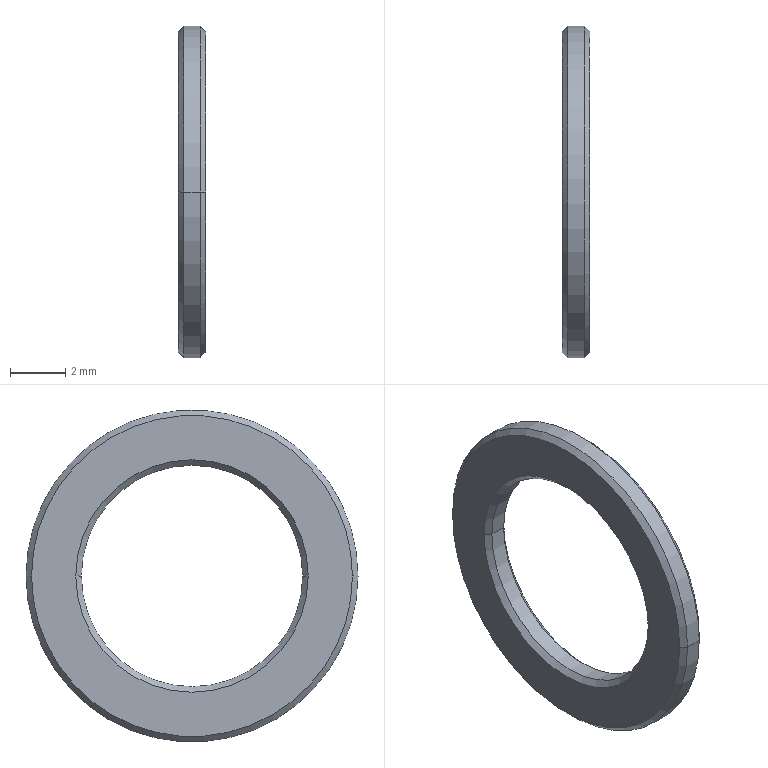Part | STEP file | 0246_017_WSSM12-8-1 | 1 solid | 14 faces | box 1 x 12 x 12 mm | volume 60.319 mm3 | cone 8 | cylinder 4 | plane 2 | commonest cylinder face diameters 8 x2 12 x2
STEP:
#1=CARTESIAN_POINT('',(0.,0.,0.));
#2=DIRECTION('',(0.,0.,1.));
#3=DIRECTION('',(1.,0.,0.));
#4=AXIS2_PLACEMENT_3D('',#1,#2,#3);
#5=CARTESIAN_POINT('',(0.2,-4.,0.));
#6=VERTEX_POINT('',#5);
#7=CARTESIAN_POINT('',(0.,-4.2,0.));
#8=VERTEX_POINT('',#7);
#9=CARTESIAN_POINT('',(0.,-4.2,0.));
#10=DIRECTION('',(-0.7071,-0.7071,0.));
#11=VECTOR('',#10,1.);
#12=LINE('',#9,#11);
#13=CARTESIAN_POINT('',(0.,0.,0.));
#14=DIRECTION('',(-1.,0.,0.));
#15=DIRECTION('',(0.,-1.,0.));
#16=AXIS2_PLACEMENT_3D('',#13,#14,#15);
#17=CONICAL_SURFACE('',#16,4.2,0.7854);
#18=CARTESIAN_POINT('',(6.283,0.));
#19=DIRECTION('',(0.,1.));
#20=VECTOR('',#19,1.);
#21=LINE('',#18,#20);
#22=(GEOMETRIC_REPRESENTATION_CONTEXT(2)PARAMETRIC_REPRESENTATION_CONTEXT()REPRESENTATION_CONTEXT('',''));
#23=DEFINITIONAL_REPRESENTATION('',(#21),#22);
#24=PCURVE('',#17,#23);
#25=CARTESIAN_POINT('',(0.,0.,0.));
#26=DIRECTION('',(-1.,0.,0.));
#27=DIRECTION('',(0.,-1.,0.));
#28=AXIS2_PLACEMENT_3D('',#25,#26,#27);
#29=CONICAL_SURFACE('',#28,4.2,0.7854);
#30=CARTESIAN_POINT('',(0.,0.));
#31=DIRECTION('',(0.,1.));
#32=VECTOR('',#31,1.);
#33=LINE('',#30,#32);
#34=(GEOMETRIC_REPRESENTATION_CONTEXT(2)PARAMETRIC_REPRESENTATION_CONTEXT()REPRESENTATION_CONTEXT('',''));
#35=DEFINITIONAL_REPRESENTATION('',(#33),#34);
#36=PCURVE('',#29,#35);
#37=SURFACE_CURVE('',#12,(#24,#36),.PCURVE_S1.);
#38=EDGE_CURVE('',#6,#8,#37,.T.);
#39=ORIENTED_EDGE('',*,*,#38,.T.);
#40=CARTESIAN_POINT('',(0.,4.2,0.));
#41=VERTEX_POINT('',#40);
#42=CARTESIAN_POINT('',(0.,0.,0.));
#43=DIRECTION('',(1.,0.,0.));
#44=DIRECTION('',(0.,-1.,0.));
#45=AXIS2_PLACEMENT_3D('',#42,#43,#44);
#46=CIRCLE('',#45,4.2);
#47=CARTESIAN_POINT('',(6.283,0.));
#48=DIRECTION('',(-1.,0.));
#49=VECTOR('',#48,1.);
#50=LINE('',#47,#49);
#51=(GEOMETRIC_REPRESENTATION_CONTEXT(2)PARAMETRIC_REPRESENTATION_CONTEXT()REPRESENTATION_CONTEXT('',''));
#52=DEFINITIONAL_REPRESENTATION('',(#50),#51);
#53=PCURVE('',#17,#52);
#54=CARTESIAN_POINT('',(0.,-5.,0.));
#55=DIRECTION('',(-1.,0.,0.));
#56=DIRECTION('',(0.,-1.,0.));
#57=AXIS2_PLACEMENT_3D('',#54,#55,#56);
#58=PLANE('',#57);
#59=CARTESIAN_POINT('',(-0.8,0.));
#60=CARTESIAN_POINT('',(-0.8,-7.275));
#61=CARTESIAN_POINT('',(-7.1,-3.637));
#62=CARTESIAN_POINT('',(-13.4,0.));
#63=CARTESIAN_POINT('',(-7.1,3.637));
#64=CARTESIAN_POINT('',(-0.8,7.275));
#65=CARTESIAN_POINT('',(-0.8,0.));
#66=(BOUNDED_CURVE()B_SPLINE_CURVE(2,(#59,#60,#61,#62,#63,#64,#65),.UNSPECIFIED.,.T.,.F.)B_SPLINE_CURVE_WITH_KNOTS((1,2,2,2,2,1),(-2.094,0.,2.094,4.189,6.283,8.378),.UNSPECIFIED.)CURVE()GEOMETRIC_REPRESENTATION_ITEM()RATIONAL_B_SPLINE_CURVE((1.,0.5,1.,0.5,1.,0.5,1.))REPRESENTATION_ITEM(''));
#67=(GEOMETRIC_REPRESENTATION_CONTEXT(2)PARAMETRIC_REPRESENTATION_CONTEXT()REPRESENTATION_CONTEXT('',''));
#68=DEFINITIONAL_REPRESENTATION('',(#66),#67);
#69=PCURVE('',#58,#68);
#70=SURFACE_CURVE('',#46,(#53,#69),.PCURVE_S1.);
#71=EDGE_CURVE('',#8,#41,#70,.T.);
#72=ORIENTED_EDGE('',*,*,#71,.T.);
#73=CARTESIAN_POINT('',(0.2,4.,0.));
#74=VERTEX_POINT('',#73);
#75=CARTESIAN_POINT('',(0.,4.2,0.));
#76=DIRECTION('',(-0.7071,0.7071,0.));
#77=VECTOR('',#76,1.);
#78=LINE('',#75,#77);
#79=CARTESIAN_POINT('',(3.142,0.));
#80=DIRECTION('',(0.,1.));
#81=VECTOR('',#80,1.);
#82=LINE('',#79,#81);
#83=(GEOMETRIC_REPRESENTATION_CONTEXT(2)PARAMETRIC_REPRESENTATION_CONTEXT()REPRESENTATION_CONTEXT('',''));
#84=DEFINITIONAL_REPRESENTATION('',(#82),#83);
#85=PCURVE('',#17,#84);
#86=CARTESIAN_POINT('',(3.142,0.));
#87=DIRECTION('',(0.,1.));
#88=VECTOR('',#87,1.);
#89=LINE('',#86,#88);
#90=(GEOMETRIC_REPRESENTATION_CONTEXT(2)PARAMETRIC_REPRESENTATION_CONTEXT()REPRESENTATION_CONTEXT('',''));
#91=DEFINITIONAL_REPRESENTATION('',(#89),#90);
#92=PCURVE('',#29,#91);
#93=SURFACE_CURVE('',#78,(#85,#92),.PCURVE_S1.);
#94=EDGE_CURVE('',#74,#41,#93,.T.);
#95=ORIENTED_EDGE('',*,*,#94,.F.);
#96=CARTESIAN_POINT('',(0.2,0.,0.));
#97=DIRECTION('',(-1.,0.,0.));
#98=DIRECTION('',(0.,-1.,0.));
#99=AXIS2_PLACEMENT_3D('',#96,#97,#98);
#100=CIRCLE('',#99,4.);
#101=CARTESIAN_POINT('',(0.,-0.2));
#102=DIRECTION('',(1.,0.));
#103=VECTOR('',#102,1.);
#104=LINE('',#101,#103);
#105=(GEOMETRIC_REPRESENTATION_CONTEXT(2)PARAMETRIC_REPRESENTATION_CONTEXT()REPRESENTATION_CONTEXT('',''));
#106=DEFINITIONAL_REPRESENTATION('',(#104),#105);
#107=PCURVE('',#17,#106);
#108=CARTESIAN_POINT('',(0.5,0.,0.));
#109=DIRECTION('',(-1.,0.,0.));
#110=DIRECTION('',(0.,-1.,0.));
#111=AXIS2_PLACEMENT_3D('',#108,#109,#110);
#112=CYLINDRICAL_SURFACE('',#111,4.);
#113=CARTESIAN_POINT('',(0.,0.3));
#114=DIRECTION('',(1.,0.));
#115=VECTOR('',#114,1.);
#116=LINE('',#113,#115);
#117=(GEOMETRIC_REPRESENTATION_CONTEXT(2)PARAMETRIC_REPRESENTATION_CONTEXT()REPRESENTATION_CONTEXT('',''));
#118=DEFINITIONAL_REPRESENTATION('',(#116),#117);
#119=PCURVE('',#112,#118);
#120=SURFACE_CURVE('',#100,(#107,#119),.PCURVE_S1.);
#121=EDGE_CURVE('',#74,#6,#120,.T.);
#122=ORIENTED_EDGE('',*,*,#121,.T.);
#123=EDGE_LOOP('',(#39,#72,#95,#122));
#124=FACE_BOUND('',#123,.F.);
#125=ADVANCED_FACE('',(#124),#17,.F.);
#126=CARTESIAN_POINT('',(0.,-5.8,0.));
#127=VERTEX_POINT('',#126);
#128=CARTESIAN_POINT('',(0.,5.8,0.));
#129=VERTEX_POINT('',#128);
#130=CARTESIAN_POINT('',(0.,0.,0.));
#131=DIRECTION('',(-1.,0.,0.));
#132=DIRECTION('',(0.,1.,0.));
#133=AXIS2_PLACEMENT_3D('',#130,#131,#132);
#134=CIRCLE('',#133,5.8);
#135=CARTESIAN_POINT('',(0.2,0.,0.));
#136=DIRECTION('',(1.,0.,0.));
#137=DIRECTION('',(0.,1.,0.));
#138=AXIS2_PLACEMENT_3D('',#135,#136,#137);
#139=CONICAL_SURFACE('',#138,6.,0.7854);
#140=CARTESIAN_POINT('',(6.283,-0.2));
#141=DIRECTION('',(-1.,0.));
#142=VECTOR('',#141,1.);
#143=LINE('',#140,#142);
#144=(GEOMETRIC_REPRESENTATION_CONTEXT(2)PARAMETRIC_REPRESENTATION_CONTEXT()REPRESENTATION_CONTEXT('',''));
#145=DEFINITIONAL_REPRESENTATION('',(#143),#144);
#146=PCURVE('',#139,#145);
#147=CARTESIAN_POINT('',(-5.,0.));
#148=DIRECTION('',(-1.,0.));
#149=AXIS2_PLACEMENT_2D('',#147,#148);
#150=CIRCLE('',#149,5.8);
#151=(GEOMETRIC_REPRESENTATION_CONTEXT(2)PARAMETRIC_REPRESENTATION_CONTEXT()REPRESENTATION_CONTEXT('',''));
#152=DEFINITIONAL_REPRESENTATION('',(#150),#151);
#153=PCURVE('',#58,#152);
#154=SURFACE_CURVE('',#134,(#146,#153),.PCURVE_S1.);
#155=EDGE_CURVE('',#127,#129,#154,.T.);
#156=ORIENTED_EDGE('',*,*,#155,.F.);
#157=CARTESIAN_POINT('',(0.2,-6.,0.));
#158=VERTEX_POINT('',#157);
#159=CARTESIAN_POINT('',(0.2,-6.,0.));
#160=DIRECTION('',(0.7071,-0.7071,0.));
#161=VECTOR('',#160,1.);
#162=LINE('',#159,#161);
#163=CARTESIAN_POINT('',(3.142,0.));
#164=DIRECTION('',(0.,1.));
#165=VECTOR('',#164,1.);
#166=LINE('',#163,#165);
#167=(GEOMETRIC_REPRESENTATION_CONTEXT(2)PARAMETRIC_REPRESENTATION_CONTEXT()REPRESENTATION_CONTEXT('',''));
#168=DEFINITIONAL_REPRESENTATION('',(#166),#167);
#169=PCURVE('',#139,#168);
#170=CARTESIAN_POINT('',(0.2,0.,0.));
#171=DIRECTION('',(1.,0.,0.));
#172=DIRECTION('',(0.,1.,0.));
#173=AXIS2_PLACEMENT_3D('',#170,#171,#172);
#174=CONICAL_SURFACE('',#173,6.,0.7854);
#175=CARTESIAN_POINT('',(3.142,0.));
#176=DIRECTION('',(0.,1.));
#177=VECTOR('',#176,1.);
#178=LINE('',#175,#177);
#179=(GEOMETRIC_REPRESENTATION_CONTEXT(2)PARAMETRIC_REPRESENTATION_CONTEXT()REPRESENTATION_CONTEXT('',''));
#180=DEFINITIONAL_REPRESENTATION('',(#178),#179);
#181=PCURVE('',#174,#180);
#182=SURFACE_CURVE('',#162,(#169,#181),.PCURVE_S1.);
#183=EDGE_CURVE('',#127,#158,#182,.T.);
#184=ORIENTED_EDGE('',*,*,#183,.T.);
#185=CARTESIAN_POINT('',(0.2,6.,0.));
#186=VERTEX_POINT('',#185);
#187=CARTESIAN_POINT('',(0.2,0.,0.));
#188=DIRECTION('',(-1.,0.,0.));
#189=DIRECTION('',(0.,-1.,0.));
#190=AXIS2_PLACEMENT_3D('',#187,#188,#189);
#191=CIRCLE('',#190,6.);
#192=CARTESIAN_POINT('',(3.142,0.));
#193=DIRECTION('',(-1.,0.));
#194=VECTOR('',#193,1.);
#195=LINE('',#192,#194);
#196=(GEOMETRIC_REPRESENTATION_CONTEXT(2)PARAMETRIC_REPRESENTATION_CONTEXT()REPRESENTATION_CONTEXT('',''));
#197=DEFINITIONAL_REPRESENTATION('',(#195),#196);
#198=PCURVE('',#139,#197);
#199=CARTESIAN_POINT('',(0.5,0.,0.));
#200=DIRECTION('',(-1.,0.,0.));
#201=DIRECTION('',(0.,-1.,0.));
#202=AXIS2_PLACEMENT_3D('',#199,#200,#201);
#203=CYLINDRICAL_SURFACE('',#202,6.);
#204=CARTESIAN_POINT('',(0.,0.3));
#205=DIRECTION('',(1.,0.));
#206=VECTOR('',#205,1.);
#207=LINE('',#204,#206);
#208=(GEOMETRIC_REPRESENTATION_CONTEXT(2)PARAMETRIC_REPRESENTATION_CONTEXT()REPRESENTATION_CONTEXT('',''));
#209=DEFINITIONAL_REPRESENTATION('',(#207),#208);
#210=PCURVE('',#203,#209);
#211=SURFACE_CURVE('',#191,(#198,#210),.PCURVE_S1.);
#212=EDGE_CURVE('',#158,#186,#211,.T.);
#213=ORIENTED_EDGE('',*,*,#212,.T.);
#214=CARTESIAN_POINT('',(0.2,6.,0.));
#215=DIRECTION('',(0.7071,0.7071,0.));
#216=VECTOR('',#215,1.);
#217=LINE('',#214,#216);
#218=CARTESIAN_POINT('',(0.,0.));
#219=DIRECTION('',(0.,1.));
#220=VECTOR('',#219,1.);
#221=LINE('',#218,#220);
#222=(GEOMETRIC_REPRESENTATION_CONTEXT(2)PARAMETRIC_REPRESENTATION_CONTEXT()REPRESENTATION_CONTEXT('',''));
#223=DEFINITIONAL_REPRESENTATION('',(#221),#222);
#224=PCURVE('',#139,#223);
#225=CARTESIAN_POINT('',(6.283,0.));
#226=DIRECTION('',(0.,1.));
#227=VECTOR('',#226,1.);
#228=LINE('',#225,#227);
#229=(GEOMETRIC_REPRESENTATION_CONTEXT(2)PARAMETRIC_REPRESENTATION_CONTEXT()REPRESENTATION_CONTEXT('',''));
#230=DEFINITIONAL_REPRESENTATION('',(#228),#229);
#231=PCURVE('',#174,#230);
#232=SURFACE_CURVE('',#217,(#224,#231),.PCURVE_S1.);
#233=EDGE_CURVE('',#129,#186,#232,.T.);
#234=ORIENTED_EDGE('',*,*,#233,.F.);
#235=EDGE_LOOP('',(#156,#184,#213,#234));
#236=FACE_BOUND('',#235,.T.);
#237=ADVANCED_FACE('',(#236),#139,.T.);
#238=CARTESIAN_POINT('',(0.8,-4.,0.));
#239=VERTEX_POINT('',#238);
#240=CARTESIAN_POINT('',(0.5,-4.,0.));
#241=DIRECTION('',(-1.,0.,0.));
#242=VECTOR('',#241,1.);
#243=LINE('',#240,#242);
#244=CARTESIAN_POINT('',(6.283,0.));
#245=DIRECTION('',(0.,1.));
#246=VECTOR('',#245,1.);
#247=LINE('',#244,#246);
#248=(GEOMETRIC_REPRESENTATION_CONTEXT(2)PARAMETRIC_REPRESENTATION_CONTEXT()REPRESENTATION_CONTEXT('',''));
#249=DEFINITIONAL_REPRESENTATION('',(#247),#248);
#250=PCURVE('',#112,#249);
#251=CARTESIAN_POINT('',(0.5,0.,0.));
#252=DIRECTION('',(-1.,0.,0.));
#253=DIRECTION('',(0.,-1.,0.));
#254=AXIS2_PLACEMENT_3D('',#251,#252,#253);
#255=CYLINDRICAL_SURFACE('',#254,4.);
#256=CARTESIAN_POINT('',(0.,0.));
#257=DIRECTION('',(0.,1.));
#258=VECTOR('',#257,1.);
#259=LINE('',#256,#258);
#260=(GEOMETRIC_REPRESENTATION_CONTEXT(2)PARAMETRIC_REPRESENTATION_CONTEXT()REPRESENTATION_CONTEXT('',''));
#261=DEFINITIONAL_REPRESENTATION('',(#259),#260);
#262=PCURVE('',#255,#261);
#263=SURFACE_CURVE('',#243,(#250,#262),.PCURVE_S1.);
#264=EDGE_CURVE('',#239,#6,#263,.T.);
#265=ORIENTED_EDGE('',*,*,#264,.T.);
#266=ORIENTED_EDGE('',*,*,#121,.F.);
#267=CARTESIAN_POINT('',(0.8,4.,0.));
#268=VERTEX_POINT('',#267);
#269=CARTESIAN_POINT('',(0.5,4.,0.));
#270=DIRECTION('',(-1.,0.,0.));
#271=VECTOR('',#270,1.);
#272=LINE('',#269,#271);
#273=CARTESIAN_POINT('',(3.142,0.));
#274=DIRECTION('',(0.,1.));
#275=VECTOR('',#274,1.);
#276=LINE('',#273,#275);
#277=(GEOMETRIC_REPRESENTATION_CONTEXT(2)PARAMETRIC_REPRESENTATION_CONTEXT()REPRESENTATION_CONTEXT('',''));
#278=DEFINITIONAL_REPRESENTATION('',(#276),#277);
#279=PCURVE('',#112,#278);
#280=CARTESIAN_POINT('',(3.142,0.));
#281=DIRECTION('',(0.,1.));
#282=VECTOR('',#281,1.);
#283=LINE('',#280,#282);
#284=(GEOMETRIC_REPRESENTATION_CONTEXT(2)PARAMETRIC_REPRESENTATION_CONTEXT()REPRESENTATION_CONTEXT('',''));
#285=DEFINITIONAL_REPRESENTATION('',(#283),#284);
#286=PCURVE('',#255,#285);
#287=SURFACE_CURVE('',#272,(#279,#286),.PCURVE_S1.);
#288=EDGE_CURVE('',#268,#74,#287,.T.);
#289=ORIENTED_EDGE('',*,*,#288,.F.);
#290=CARTESIAN_POINT('',(0.8,0.,0.));
#291=DIRECTION('',(-1.,0.,0.));
#292=DIRECTION('',(0.,-1.,0.));
#293=AXIS2_PLACEMENT_3D('',#290,#291,#292);
#294=CIRCLE('',#293,4.);
#295=CARTESIAN_POINT('',(0.,-0.3));
#296=DIRECTION('',(1.,0.));
#297=VECTOR('',#296,1.);
#298=LINE('',#295,#297);
#299=(GEOMETRIC_REPRESENTATION_CONTEXT(2)PARAMETRIC_REPRESENTATION_CONTEXT()REPRESENTATION_CONTEXT('',''));
#300=DEFINITIONAL_REPRESENTATION('',(#298),#299);
#301=PCURVE('',#112,#300);
#302=CARTESIAN_POINT('',(1.,0.,0.));
#303=DIRECTION('',(1.,0.,0.));
#304=DIRECTION('',(0.,1.,0.));
#305=AXIS2_PLACEMENT_3D('',#302,#303,#304);
#306=CONICAL_SURFACE('',#305,4.2,0.7854);
#307=CARTESIAN_POINT('',(9.425,-0.2));
#308=DIRECTION('',(-1.,0.));
#309=VECTOR('',#308,1.);
#310=LINE('',#307,#309);
#311=(GEOMETRIC_REPRESENTATION_CONTEXT(2)PARAMETRIC_REPRESENTATION_CONTEXT()REPRESENTATION_CONTEXT('',''));
#312=DEFINITIONAL_REPRESENTATION('',(#310),#311);
#313=PCURVE('',#306,#312);
#314=SURFACE_CURVE('',#294,(#301,#313),.PCURVE_S1.);
#315=EDGE_CURVE('',#268,#239,#314,.T.);
#316=ORIENTED_EDGE('',*,*,#315,.T.);
#317=EDGE_LOOP('',(#265,#266,#289,#316));
#318=FACE_BOUND('',#317,.F.);
#319=ADVANCED_FACE('',(#318),#112,.F.);
#320=CARTESIAN_POINT('',(0.8,-6.,0.));
#321=VERTEX_POINT('',#320);
#322=CARTESIAN_POINT('',(0.8,6.,0.));
#323=VERTEX_POINT('',#322);
#324=CARTESIAN_POINT('',(0.8,0.,0.));
#325=DIRECTION('',(-1.,0.,0.));
#326=DIRECTION('',(0.,-1.,0.));
#327=AXIS2_PLACEMENT_3D('',#324,#325,#326);
#328=CIRCLE('',#327,6.);
#329=CARTESIAN_POINT('',(0.,-0.3));
#330=DIRECTION('',(1.,0.));
#331=VECTOR('',#330,1.);
#332=LINE('',#329,#331);
#333=(GEOMETRIC_REPRESENTATION_CONTEXT(2)PARAMETRIC_REPRESENTATION_CONTEXT()REPRESENTATION_CONTEXT('',''));
#334=DEFINITIONAL_REPRESENTATION('',(#332),#333);
#335=PCURVE('',#203,#334);
#336=CARTESIAN_POINT('',(0.8,0.,0.));
#337=DIRECTION('',(-1.,0.,0.));
#338=DIRECTION('',(0.,-1.,0.));
#339=AXIS2_PLACEMENT_3D('',#336,#337,#338);
#340=CONICAL_SURFACE('',#339,6.,0.7854);
#341=CARTESIAN_POINT('',(0.,0.));
#342=DIRECTION('',(1.,0.));
#343=VECTOR('',#342,1.);
#344=LINE('',#341,#343);
#345=(GEOMETRIC_REPRESENTATION_CONTEXT(2)PARAMETRIC_REPRESENTATION_CONTEXT()REPRESENTATION_CONTEXT('',''));
#346=DEFINITIONAL_REPRESENTATION('',(#344),#345);
#347=PCURVE('',#340,#346);
#348=SURFACE_CURVE('',#328,(#335,#347),.PCURVE_S1.);
#349=EDGE_CURVE('',#321,#323,#348,.T.);
#350=ORIENTED_EDGE('',*,*,#349,.T.);
#351=CARTESIAN_POINT('',(0.5,6.,0.));
#352=DIRECTION('',(-1.,0.,0.));
#353=VECTOR('',#352,1.);
#354=LINE('',#351,#353);
#355=CARTESIAN_POINT('',(3.142,0.));
#356=DIRECTION('',(0.,1.));
#357=VECTOR('',#356,1.);
#358=LINE('',#355,#357);
#359=(GEOMETRIC_REPRESENTATION_CONTEXT(2)PARAMETRIC_REPRESENTATION_CONTEXT()REPRESENTATION_CONTEXT('',''));
#360=DEFINITIONAL_REPRESENTATION('',(#358),#359);
#361=PCURVE('',#203,#360);
#362=CARTESIAN_POINT('',(0.5,0.,0.));
#363=DIRECTION('',(-1.,0.,0.));
#364=DIRECTION('',(0.,-1.,0.));
#365=AXIS2_PLACEMENT_3D('',#362,#363,#364);
#366=CYLINDRICAL_SURFACE('',#365,6.);
#367=CARTESIAN_POINT('',(3.142,0.));
#368=DIRECTION('',(0.,1.));
#369=VECTOR('',#368,1.);
#370=LINE('',#367,#369);
#371=(GEOMETRIC_REPRESENTATION_CONTEXT(2)PARAMETRIC_REPRESENTATION_CONTEXT()REPRESENTATION_CONTEXT('',''));
#372=DEFINITIONAL_REPRESENTATION('',(#370),#371);
#373=PCURVE('',#366,#372);
#374=SURFACE_CURVE('',#354,(#361,#373),.PCURVE_S1.);
#375=EDGE_CURVE('',#323,#186,#374,.T.);
#376=ORIENTED_EDGE('',*,*,#375,.T.);
#377=ORIENTED_EDGE('',*,*,#212,.F.);
#378=CARTESIAN_POINT('',(0.5,-6.,0.));
#379=DIRECTION('',(-1.,0.,0.));
#380=VECTOR('',#379,1.);
#381=LINE('',#378,#380);
#382=CARTESIAN_POINT('',(0.,0.));
#383=DIRECTION('',(0.,1.));
#384=VECTOR('',#383,1.);
#385=LINE('',#382,#384);
#386=(GEOMETRIC_REPRESENTATION_CONTEXT(2)PARAMETRIC_REPRESENTATION_CONTEXT()REPRESENTATION_CONTEXT('',''));
#387=DEFINITIONAL_REPRESENTATION('',(#385),#386);
#388=PCURVE('',#203,#387);
#389=CARTESIAN_POINT('',(6.283,0.));
#390=DIRECTION('',(0.,1.));
#391=VECTOR('',#390,1.);
#392=LINE('',#389,#391);
#393=(GEOMETRIC_REPRESENTATION_CONTEXT(2)PARAMETRIC_REPRESENTATION_CONTEXT()REPRESENTATION_CONTEXT('',''));
#394=DEFINITIONAL_REPRESENTATION('',(#392),#393);
#395=PCURVE('',#366,#394);
#396=SURFACE_CURVE('',#381,(#388,#395),.PCURVE_S1.);
#397=EDGE_CURVE('',#321,#158,#396,.T.);
#398=ORIENTED_EDGE('',*,*,#397,.F.);
#399=EDGE_LOOP('',(#350,#376,#377,#398));
#400=FACE_BOUND('',#399,.T.);
#401=ADVANCED_FACE('',(#400),#203,.T.);
#402=CARTESIAN_POINT('',(1.,4.2,0.));
#403=VERTEX_POINT('',#402);
#404=CARTESIAN_POINT('',(1.,4.2,0.));
#405=DIRECTION('',(0.7071,0.7071,0.));
#406=VECTOR('',#405,1.);
#407=LINE('',#404,#406);
#408=CARTESIAN_POINT('',(6.283,0.));
#409=DIRECTION('',(0.,1.));
#410=VECTOR('',#409,1.);
#411=LINE('',#408,#410);
#412=(GEOMETRIC_REPRESENTATION_CONTEXT(2)PARAMETRIC_REPRESENTATION_CONTEXT()REPRESENTATION_CONTEXT('',''));
#413=DEFINITIONAL_REPRESENTATION('',(#411),#412);
#414=PCURVE('',#306,#413);
#415=CARTESIAN_POINT('',(1.,0.,0.));
#416=DIRECTION('',(1.,0.,0.));
#417=DIRECTION('',(0.,1.,0.));
#418=AXIS2_PLACEMENT_3D('',#415,#416,#417);
#419=CONICAL_SURFACE('',#418,4.2,0.7854);
#420=CARTESIAN_POINT('',(0.,0.));
#421=DIRECTION('',(0.,1.));
#422=VECTOR('',#421,1.);
#423=LINE('',#420,#422);
#424=(GEOMETRIC_REPRESENTATION_CONTEXT(2)PARAMETRIC_REPRESENTATION_CONTEXT()REPRESENTATION_CONTEXT('',''));
#425=DEFINITIONAL_REPRESENTATION('',(#423),#424);
#426=PCURVE('',#419,#425);
#427=SURFACE_CURVE('',#407,(#414,#426),.PCURVE_S1.);
#428=EDGE_CURVE('',#268,#403,#427,.T.);
#429=ORIENTED_EDGE('',*,*,#428,.T.);
#430=CARTESIAN_POINT('',(1.,-4.2,0.));
#431=VERTEX_POINT('',#430);
#432=CARTESIAN_POINT('',(1.,0.,0.));
#433=DIRECTION('',(-1.,0.,0.));
#434=DIRECTION('',(0.,1.,0.));
#435=AXIS2_PLACEMENT_3D('',#432,#433,#434);
#436=CIRCLE('',#435,4.2);
#437=CARTESIAN_POINT('',(6.283,0.));
#438=DIRECTION('',(-1.,0.));
#439=VECTOR('',#438,1.);
#440=LINE('',#437,#439);
#441=(GEOMETRIC_REPRESENTATION_CONTEXT(2)PARAMETRIC_REPRESENTATION_CONTEXT()REPRESENTATION_CONTEXT('',''));
#442=DEFINITIONAL_REPRESENTATION('',(#440),#441);
#443=PCURVE('',#306,#442);
#444=CARTESIAN_POINT('',(1.,-5.,0.));
#445=DIRECTION('',(1.,0.,0.));
#446=DIRECTION('',(0.,1.,0.));
#447=AXIS2_PLACEMENT_3D('',#444,#445,#446);
#448=PLANE('',#447);
#449=CARTESIAN_POINT('',(9.2,0.));
#450=CARTESIAN_POINT('',(9.2,-7.275));
#451=CARTESIAN_POINT('',(2.9,-3.637));
#452=CARTESIAN_POINT('',(-3.4,0.));
#453=CARTESIAN_POINT('',(2.9,3.637));
#454=CARTESIAN_POINT('',(9.2,7.275));
#455=CARTESIAN_POINT('',(9.2,0.));
#456=(BOUNDED_CURVE()B_SPLINE_CURVE(2,(#449,#450,#451,#452,#453,#454,#455),.UNSPECIFIED.,.T.,.F.)B_SPLINE_CURVE_WITH_KNOTS((1,2,2,2,2,1),(-2.094,0.,2.094,4.189,6.283,8.378),.UNSPECIFIED.)CURVE()GEOMETRIC_REPRESENTATION_ITEM()RATIONAL_B_SPLINE_CURVE((1.,0.5,1.,0.5,1.,0.5,1.))REPRESENTATION_ITEM(''));
#457=(GEOMETRIC_REPRESENTATION_CONTEXT(2)PARAMETRIC_REPRESENTATION_CONTEXT()REPRESENTATION_CONTEXT('',''));
#458=DEFINITIONAL_REPRESENTATION('',(#456),#457);
#459=PCURVE('',#448,#458);
#460=SURFACE_CURVE('',#436,(#443,#459),.PCURVE_S1.);
#461=EDGE_CURVE('',#403,#431,#460,.T.);
#462=ORIENTED_EDGE('',*,*,#461,.T.);
#463=CARTESIAN_POINT('',(1.,-4.2,0.));
#464=DIRECTION('',(0.7071,-0.7071,0.));
#465=VECTOR('',#464,1.);
#466=LINE('',#463,#465);
#467=CARTESIAN_POINT('',(3.142,0.));
#468=DIRECTION('',(0.,1.));
#469=VECTOR('',#468,1.);
#470=LINE('',#467,#469);
#471=(GEOMETRIC_REPRESENTATION_CONTEXT(2)PARAMETRIC_REPRESENTATION_CONTEXT()REPRESENTATION_CONTEXT('',''));
#472=DEFINITIONAL_REPRESENTATION('',(#470),#471);
#473=PCURVE('',#306,#472);
#474=CARTESIAN_POINT('',(3.142,0.));
#475=DIRECTION('',(0.,1.));
#476=VECTOR('',#475,1.);
#477=LINE('',#474,#476);
#478=(GEOMETRIC_REPRESENTATION_CONTEXT(2)PARAMETRIC_REPRESENTATION_CONTEXT()REPRESENTATION_CONTEXT('',''));
#479=DEFINITIONAL_REPRESENTATION('',(#477),#478);
#480=PCURVE('',#419,#479);
#481=SURFACE_CURVE('',#466,(#473,#480),.PCURVE_S1.);
#482=EDGE_CURVE('',#239,#431,#481,.T.);
#483=ORIENTED_EDGE('',*,*,#482,.F.);
#484=ORIENTED_EDGE('',*,*,#315,.F.);
#485=EDGE_LOOP('',(#429,#462,#483,#484));
#486=FACE_BOUND('',#485,.F.);
#487=ADVANCED_FACE('',(#486),#306,.F.);
#488=CARTESIAN_POINT('',(1.,-5.8,0.));
#489=VERTEX_POINT('',#488);
#490=CARTESIAN_POINT('',(1.,5.8,0.));
#491=VERTEX_POINT('',#490);
#492=CARTESIAN_POINT('',(1.,0.,0.));
#493=DIRECTION('',(-1.,0.,0.));
#494=DIRECTION('',(0.,-1.,0.));
#495=AXIS2_PLACEMENT_3D('',#492,#493,#494);
#496=CIRCLE('',#495,5.8);
#497=CARTESIAN_POINT('',(0.,-0.2));
#498=DIRECTION('',(1.,0.));
#499=VECTOR('',#498,1.);
#500=LINE('',#497,#499);
#501=(GEOMETRIC_REPRESENTATION_CONTEXT(2)PARAMETRIC_REPRESENTATION_CONTEXT()REPRESENTATION_CONTEXT('',''));
#502=DEFINITIONAL_REPRESENTATION('',(#500),#501);
#503=PCURVE('',#340,#502);
#504=CARTESIAN_POINT('',(-0.8,0.));
#505=CARTESIAN_POINT('',(-0.8,10.046));
#506=CARTESIAN_POINT('',(7.9,5.023));
#507=CARTESIAN_POINT('',(16.6,0.));
#508=CARTESIAN_POINT('',(7.9,-5.023));
#509=CARTESIAN_POINT('',(-0.8,-10.046));
#510=CARTESIAN_POINT('',(-0.8,0.));
#511=(BOUNDED_CURVE()B_SPLINE_CURVE(2,(#504,#505,#506,#507,#508,#509,#510),.UNSPECIFIED.,.T.,.F.)B_SPLINE_CURVE_WITH_KNOTS((1,2,2,2,2,1),(-2.094,0.,2.094,4.189,6.283,8.378),.UNSPECIFIED.)CURVE()GEOMETRIC_REPRESENTATION_ITEM()RATIONAL_B_SPLINE_CURVE((1.,0.5,1.,0.5,1.,0.5,1.))REPRESENTATION_ITEM(''));
#512=(GEOMETRIC_REPRESENTATION_CONTEXT(2)PARAMETRIC_REPRESENTATION_CONTEXT()REPRESENTATION_CONTEXT('',''));
#513=DEFINITIONAL_REPRESENTATION('',(#511),#512);
#514=PCURVE('',#448,#513);
#515=SURFACE_CURVE('',#496,(#503,#514),.PCURVE_S1.);
#516=EDGE_CURVE('',#489,#491,#515,.T.);
#517=ORIENTED_EDGE('',*,*,#516,.T.);
#518=CARTESIAN_POINT('',(0.8,6.,0.));
#519=DIRECTION('',(-0.7071,0.7071,0.));
#520=VECTOR('',#519,1.);
#521=LINE('',#518,#520);
#522=CARTESIAN_POINT('',(3.142,0.));
#523=DIRECTION('',(0.,1.));
#524=VECTOR('',#523,1.);
#525=LINE('',#522,#524);
#526=(GEOMETRIC_REPRESENTATION_CONTEXT(2)PARAMETRIC_REPRESENTATION_CONTEXT()REPRESENTATION_CONTEXT('',''));
#527=DEFINITIONAL_REPRESENTATION('',(#525),#526);
#528=PCURVE('',#340,#527);
#529=CARTESIAN_POINT('',(0.8,0.,0.));
#530=DIRECTION('',(-1.,0.,0.));
#531=DIRECTION('',(0.,-1.,0.));
#532=AXIS2_PLACEMENT_3D('',#529,#530,#531);
#533=CONICAL_SURFACE('',#532,6.,0.7854);
#534=CARTESIAN_POINT('',(3.142,0.));
#535=DIRECTION('',(0.,1.));
#536=VECTOR('',#535,1.);
#537=LINE('',#534,#536);
#538=(GEOMETRIC_REPRESENTATION_CONTEXT(2)PARAMETRIC_REPRESENTATION_CONTEXT()REPRESENTATION_CONTEXT('',''));
#539=DEFINITIONAL_REPRESENTATION('',(#537),#538);
#540=PCURVE('',#533,#539);
#541=SURFACE_CURVE('',#521,(#528,#540),.PCURVE_S1.);
#542=EDGE_CURVE('',#491,#323,#541,.T.);
#543=ORIENTED_EDGE('',*,*,#542,.T.);
#544=ORIENTED_EDGE('',*,*,#349,.F.);
#545=CARTESIAN_POINT('',(0.8,-6.,0.));
#546=DIRECTION('',(-0.7071,-0.7071,0.));
#547=VECTOR('',#546,1.);
#548=LINE('',#545,#547);
#549=CARTESIAN_POINT('',(0.,0.));
#550=DIRECTION('',(0.,1.));
#551=VECTOR('',#550,1.);
#552=LINE('',#549,#551);
#553=(GEOMETRIC_REPRESENTATION_CONTEXT(2)PARAMETRIC_REPRESENTATION_CONTEXT()REPRESENTATION_CONTEXT('',''));
#554=DEFINITIONAL_REPRESENTATION('',(#552),#553);
#555=PCURVE('',#340,#554);
#556=CARTESIAN_POINT('',(6.283,0.));
#557=DIRECTION('',(0.,1.));
#558=VECTOR('',#557,1.);
#559=LINE('',#556,#558);
#560=(GEOMETRIC_REPRESENTATION_CONTEXT(2)PARAMETRIC_REPRESENTATION_CONTEXT()REPRESENTATION_CONTEXT('',''));
#561=DEFINITIONAL_REPRESENTATION('',(#559),#560);
#562=PCURVE('',#533,#561);
#563=SURFACE_CURVE('',#548,(#555,#562),.PCURVE_S1.);
#564=EDGE_CURVE('',#489,#321,#563,.T.);
#565=ORIENTED_EDGE('',*,*,#564,.F.);
#566=EDGE_LOOP('',(#517,#543,#544,#565));
#567=FACE_BOUND('',#566,.T.);
#568=ADVANCED_FACE('',(#567),#340,.T.);
#569=ORIENTED_EDGE('',*,*,#71,.T.);
#570=CARTESIAN_POINT('',(0.,0.,0.));
#571=DIRECTION('',(1.,0.,0.));
#572=DIRECTION('',(0.,-1.,0.));
#573=AXIS2_PLACEMENT_3D('',#570,#571,#572);
#574=CIRCLE('',#573,4.2);
#575=CARTESIAN_POINT('',(-0.8,0.));
#576=CARTESIAN_POINT('',(-0.8,-7.275));
#577=CARTESIAN_POINT('',(-7.1,-3.637));
#578=CARTESIAN_POINT('',(-13.4,0.));
#579=CARTESIAN_POINT('',(-7.1,3.637));
#580=CARTESIAN_POINT('',(-0.8,7.275));
#581=CARTESIAN_POINT('',(-0.8,0.));
#582=(BOUNDED_CURVE()B_SPLINE_CURVE(2,(#575,#576,#577,#578,#579,#580,#581),.UNSPECIFIED.,.T.,.F.)B_SPLINE_CURVE_WITH_KNOTS((1,2,2,2,2,1),(-2.094,0.,2.094,4.189,6.283,8.378),.UNSPECIFIED.)CURVE()GEOMETRIC_REPRESENTATION_ITEM()RATIONAL_B_SPLINE_CURVE((1.,0.5,1.,0.5,1.,0.5,1.))REPRESENTATION_ITEM(''));
#583=(GEOMETRIC_REPRESENTATION_CONTEXT(2)PARAMETRIC_REPRESENTATION_CONTEXT()REPRESENTATION_CONTEXT('',''));
#584=DEFINITIONAL_REPRESENTATION('',(#582),#583);
#585=PCURVE('',#58,#584);
#586=CARTESIAN_POINT('',(6.283,0.));
#587=DIRECTION('',(-1.,0.));
#588=VECTOR('',#587,1.);
#589=LINE('',#586,#588);
#590=(GEOMETRIC_REPRESENTATION_CONTEXT(2)PARAMETRIC_REPRESENTATION_CONTEXT()REPRESENTATION_CONTEXT('',''));
#591=DEFINITIONAL_REPRESENTATION('',(#589),#590);
#592=PCURVE('',#29,#591);
#593=SURFACE_CURVE('',#574,(#585,#592),.PCURVE_S1.);
#594=EDGE_CURVE('',#41,#8,#593,.T.);
#595=ORIENTED_EDGE('',*,*,#594,.T.);
#596=EDGE_LOOP('',(#569,#595));
#597=FACE_BOUND('',#596,.T.);
#598=CARTESIAN_POINT('',(0.,0.,0.));
#599=DIRECTION('',(-1.,0.,0.));
#600=DIRECTION('',(0.,1.,0.));
#601=AXIS2_PLACEMENT_3D('',#598,#599,#600);
#602=CIRCLE('',#601,5.8);
#603=CARTESIAN_POINT('',(-5.,0.));
#604=DIRECTION('',(-1.,0.));
#605=AXIS2_PLACEMENT_2D('',#603,#604);
#606=CIRCLE('',#605,5.8);
#607=(GEOMETRIC_REPRESENTATION_CONTEXT(2)PARAMETRIC_REPRESENTATION_CONTEXT()REPRESENTATION_CONTEXT('',''));
#608=DEFINITIONAL_REPRESENTATION('',(#606),#607);
#609=PCURVE('',#58,#608);
#610=CARTESIAN_POINT('',(6.283,-0.2));
#611=DIRECTION('',(-1.,0.));
#612=VECTOR('',#611,1.);
#613=LINE('',#610,#612);
#614=(GEOMETRIC_REPRESENTATION_CONTEXT(2)PARAMETRIC_REPRESENTATION_CONTEXT()REPRESENTATION_CONTEXT('',''));
#615=DEFINITIONAL_REPRESENTATION('',(#613),#614);
#616=PCURVE('',#174,#615);
#617=SURFACE_CURVE('',#602,(#609,#616),.PCURVE_S1.);
#618=EDGE_CURVE('',#129,#127,#617,.T.);
#619=ORIENTED_EDGE('',*,*,#618,.T.);
#620=ORIENTED_EDGE('',*,*,#155,.T.);
#621=EDGE_LOOP('',(#619,#620));
#622=FACE_BOUND('',#621,.T.);
#623=ADVANCED_FACE('',(#597,#622),#58,.T.);
#624=ORIENTED_EDGE('',*,*,#594,.T.);
#625=ORIENTED_EDGE('',*,*,#38,.F.);
#626=CARTESIAN_POINT('',(0.2,0.,0.));
#627=DIRECTION('',(-1.,0.,0.));
#628=DIRECTION('',(0.,-1.,0.));
#629=AXIS2_PLACEMENT_3D('',#626,#627,#628);
#630=CIRCLE('',#629,4.);
#631=CARTESIAN_POINT('',(0.,-0.2));
#632=DIRECTION('',(1.,0.));
#633=VECTOR('',#632,1.);
#634=LINE('',#631,#633);
#635=(GEOMETRIC_REPRESENTATION_CONTEXT(2)PARAMETRIC_REPRESENTATION_CONTEXT()REPRESENTATION_CONTEXT('',''));
#636=DEFINITIONAL_REPRESENTATION('',(#634),#635);
#637=PCURVE('',#29,#636);
#638=CARTESIAN_POINT('',(0.,0.3));
#639=DIRECTION('',(1.,0.));
#640=VECTOR('',#639,1.);
#641=LINE('',#638,#640);
#642=(GEOMETRIC_REPRESENTATION_CONTEXT(2)PARAMETRIC_REPRESENTATION_CONTEXT()REPRESENTATION_CONTEXT('',''));
#643=DEFINITIONAL_REPRESENTATION('',(#641),#642);
#644=PCURVE('',#255,#643);
#645=SURFACE_CURVE('',#630,(#637,#644),.PCURVE_S1.);
#646=EDGE_CURVE('',#6,#74,#645,.T.);
#647=ORIENTED_EDGE('',*,*,#646,.T.);
#648=ORIENTED_EDGE('',*,*,#94,.T.);
#649=EDGE_LOOP('',(#624,#625,#647,#648));
#650=FACE_BOUND('',#649,.F.);
#651=ADVANCED_FACE('',(#650),#29,.F.);
#652=ORIENTED_EDGE('',*,*,#183,.F.);
#653=ORIENTED_EDGE('',*,*,#618,.F.);
#654=ORIENTED_EDGE('',*,*,#233,.T.);
#655=CARTESIAN_POINT('',(0.2,0.,0.));
#656=DIRECTION('',(-1.,0.,0.));
#657=DIRECTION('',(0.,-1.,0.));
#658=AXIS2_PLACEMENT_3D('',#655,#656,#657);
#659=CIRCLE('',#658,6.);
#660=CARTESIAN_POINT('',(9.425,0.));
#661=DIRECTION('',(-1.,0.));
#662=VECTOR('',#661,1.);
#663=LINE('',#660,#662);
#664=(GEOMETRIC_REPRESENTATION_CONTEXT(2)PARAMETRIC_REPRESENTATION_CONTEXT()REPRESENTATION_CONTEXT('',''));
#665=DEFINITIONAL_REPRESENTATION('',(#663),#664);
#666=PCURVE('',#174,#665);
#667=CARTESIAN_POINT('',(0.,0.3));
#668=DIRECTION('',(1.,0.));
#669=VECTOR('',#668,1.);
#670=LINE('',#667,#669);
#671=(GEOMETRIC_REPRESENTATION_CONTEXT(2)PARAMETRIC_REPRESENTATION_CONTEXT()REPRESENTATION_CONTEXT('',''));
#672=DEFINITIONAL_REPRESENTATION('',(#670),#671);
#673=PCURVE('',#366,#672);
#674=SURFACE_CURVE('',#659,(#666,#673),.PCURVE_S1.);
#675=EDGE_CURVE('',#186,#158,#674,.T.);
#676=ORIENTED_EDGE('',*,*,#675,.T.);
#677=EDGE_LOOP('',(#652,#653,#654,#676));
#678=FACE_BOUND('',#677,.T.);
#679=ADVANCED_FACE('',(#678),#174,.T.);
#680=ORIENTED_EDGE('',*,*,#646,.F.);
#681=ORIENTED_EDGE('',*,*,#264,.F.);
#682=CARTESIAN_POINT('',(0.8,0.,0.));
#683=DIRECTION('',(-1.,0.,0.));
#684=DIRECTION('',(0.,-1.,0.));
#685=AXIS2_PLACEMENT_3D('',#682,#683,#684);
#686=CIRCLE('',#685,4.);
#687=CARTESIAN_POINT('',(0.,-0.3));
#688=DIRECTION('',(1.,0.));
#689=VECTOR('',#688,1.);
#690=LINE('',#687,#689);
#691=(GEOMETRIC_REPRESENTATION_CONTEXT(2)PARAMETRIC_REPRESENTATION_CONTEXT()REPRESENTATION_CONTEXT('',''));
#692=DEFINITIONAL_REPRESENTATION('',(#690),#691);
#693=PCURVE('',#255,#692);
#694=CARTESIAN_POINT('',(3.142,-0.2));
#695=DIRECTION('',(-1.,0.));
#696=VECTOR('',#695,1.);
#697=LINE('',#694,#696);
#698=(GEOMETRIC_REPRESENTATION_CONTEXT(2)PARAMETRIC_REPRESENTATION_CONTEXT()REPRESENTATION_CONTEXT('',''));
#699=DEFINITIONAL_REPRESENTATION('',(#697),#698);
#700=PCURVE('',#419,#699);
#701=SURFACE_CURVE('',#686,(#693,#700),.PCURVE_S1.);
#702=EDGE_CURVE('',#239,#268,#701,.T.);
#703=ORIENTED_EDGE('',*,*,#702,.T.);
#704=ORIENTED_EDGE('',*,*,#288,.T.);
#705=EDGE_LOOP('',(#680,#681,#703,#704));
#706=FACE_BOUND('',#705,.F.);
#707=ADVANCED_FACE('',(#706),#255,.F.);
#708=ORIENTED_EDGE('',*,*,#375,.F.);
#709=CARTESIAN_POINT('',(0.8,0.,0.));
#710=DIRECTION('',(-1.,0.,0.));
#711=DIRECTION('',(0.,-1.,0.));
#712=AXIS2_PLACEMENT_3D('',#709,#710,#711);
#713=CIRCLE('',#712,6.);
#714=CARTESIAN_POINT('',(0.,-0.3));
#715=DIRECTION('',(1.,0.));
#716=VECTOR('',#715,1.);
#717=LINE('',#714,#716);
#718=(GEOMETRIC_REPRESENTATION_CONTEXT(2)PARAMETRIC_REPRESENTATION_CONTEXT()REPRESENTATION_CONTEXT('',''));
#719=DEFINITIONAL_REPRESENTATION('',(#717),#718);
#720=PCURVE('',#366,#719);
#721=CARTESIAN_POINT('',(0.,0.));
#722=DIRECTION('',(1.,0.));
#723=VECTOR('',#722,1.);
#724=LINE('',#721,#723);
#725=(GEOMETRIC_REPRESENTATION_CONTEXT(2)PARAMETRIC_REPRESENTATION_CONTEXT()REPRESENTATION_CONTEXT('',''));
#726=DEFINITIONAL_REPRESENTATION('',(#724),#725);
#727=PCURVE('',#533,#726);
#728=SURFACE_CURVE('',#713,(#720,#727),.PCURVE_S1.);
#729=EDGE_CURVE('',#323,#321,#728,.T.);
#730=ORIENTED_EDGE('',*,*,#729,.T.);
#731=ORIENTED_EDGE('',*,*,#397,.T.);
#732=ORIENTED_EDGE('',*,*,#675,.F.);
#733=EDGE_LOOP('',(#708,#730,#731,#732));
#734=FACE_BOUND('',#733,.T.);
#735=ADVANCED_FACE('',(#734),#366,.T.);
#736=CARTESIAN_POINT('',(1.,0.,0.));
#737=DIRECTION('',(-1.,0.,0.));
#738=DIRECTION('',(0.,1.,0.));
#739=AXIS2_PLACEMENT_3D('',#736,#737,#738);
#740=CIRCLE('',#739,4.2);
#741=CARTESIAN_POINT('',(6.283,0.));
#742=DIRECTION('',(-1.,0.));
#743=VECTOR('',#742,1.);
#744=LINE('',#741,#743);
#745=(GEOMETRIC_REPRESENTATION_CONTEXT(2)PARAMETRIC_REPRESENTATION_CONTEXT()REPRESENTATION_CONTEXT('',''));
#746=DEFINITIONAL_REPRESENTATION('',(#744),#745);
#747=PCURVE('',#419,#746);
#748=CARTESIAN_POINT('',(9.2,0.));
#749=CARTESIAN_POINT('',(9.2,-7.275));
#750=CARTESIAN_POINT('',(2.9,-3.637));
#751=CARTESIAN_POINT('',(-3.4,0.));
#752=CARTESIAN_POINT('',(2.9,3.637));
#753=CARTESIAN_POINT('',(9.2,7.275));
#754=CARTESIAN_POINT('',(9.2,0.));
#755=(BOUNDED_CURVE()B_SPLINE_CURVE(2,(#748,#749,#750,#751,#752,#753,#754),.UNSPECIFIED.,.T.,.F.)B_SPLINE_CURVE_WITH_KNOTS((1,2,2,2,2,1),(-2.094,0.,2.094,4.189,6.283,8.378),.UNSPECIFIED.)CURVE()GEOMETRIC_REPRESENTATION_ITEM()RATIONAL_B_SPLINE_CURVE((1.,0.5,1.,0.5,1.,0.5,1.))REPRESENTATION_ITEM(''));
#756=(GEOMETRIC_REPRESENTATION_CONTEXT(2)PARAMETRIC_REPRESENTATION_CONTEXT()REPRESENTATION_CONTEXT('',''));
#757=DEFINITIONAL_REPRESENTATION('',(#755),#756);
#758=PCURVE('',#448,#757);
#759=SURFACE_CURVE('',#740,(#747,#758),.PCURVE_S1.);
#760=EDGE_CURVE('',#431,#403,#759,.T.);
#761=ORIENTED_EDGE('',*,*,#760,.T.);
#762=ORIENTED_EDGE('',*,*,#428,.F.);
#763=ORIENTED_EDGE('',*,*,#702,.F.);
#764=ORIENTED_EDGE('',*,*,#482,.T.);
#765=EDGE_LOOP('',(#761,#762,#763,#764));
#766=FACE_BOUND('',#765,.F.);
#767=ADVANCED_FACE('',(#766),#419,.F.);
#768=ORIENTED_EDGE('',*,*,#542,.F.);
#769=CARTESIAN_POINT('',(1.,0.,0.));
#770=DIRECTION('',(-1.,0.,0.));
#771=DIRECTION('',(0.,-1.,0.));
#772=AXIS2_PLACEMENT_3D('',#769,#770,#771);
#773=CIRCLE('',#772,5.8);
#774=CARTESIAN_POINT('',(0.,-0.2));
#775=DIRECTION('',(1.,0.));
#776=VECTOR('',#775,1.);
#777=LINE('',#774,#776);
#778=(GEOMETRIC_REPRESENTATION_CONTEXT(2)PARAMETRIC_REPRESENTATION_CONTEXT()REPRESENTATION_CONTEXT('',''));
#779=DEFINITIONAL_REPRESENTATION('',(#777),#778);
#780=PCURVE('',#533,#779);
#781=CARTESIAN_POINT('',(-0.8,0.));
#782=CARTESIAN_POINT('',(-0.8,10.046));
#783=CARTESIAN_POINT('',(7.9,5.023));
#784=CARTESIAN_POINT('',(16.6,0.));
#785=CARTESIAN_POINT('',(7.9,-5.023));
#786=CARTESIAN_POINT('',(-0.8,-10.046));
#787=CARTESIAN_POINT('',(-0.8,0.));
#788=(BOUNDED_CURVE()B_SPLINE_CURVE(2,(#781,#782,#783,#784,#785,#786,#787),.UNSPECIFIED.,.T.,.F.)B_SPLINE_CURVE_WITH_KNOTS((1,2,2,2,2,1),(-2.094,0.,2.094,4.189,6.283,8.378),.UNSPECIFIED.)CURVE()GEOMETRIC_REPRESENTATION_ITEM()RATIONAL_B_SPLINE_CURVE((1.,0.5,1.,0.5,1.,0.5,1.))REPRESENTATION_ITEM(''));
#789=(GEOMETRIC_REPRESENTATION_CONTEXT(2)PARAMETRIC_REPRESENTATION_CONTEXT()REPRESENTATION_CONTEXT('',''));
#790=DEFINITIONAL_REPRESENTATION('',(#788),#789);
#791=PCURVE('',#448,#790);
#792=SURFACE_CURVE('',#773,(#780,#791),.PCURVE_S1.);
#793=EDGE_CURVE('',#491,#489,#792,.T.);
#794=ORIENTED_EDGE('',*,*,#793,.T.);
#795=ORIENTED_EDGE('',*,*,#564,.T.);
#796=ORIENTED_EDGE('',*,*,#729,.F.);
#797=EDGE_LOOP('',(#768,#794,#795,#796));
#798=FACE_BOUND('',#797,.T.);
#799=ADVANCED_FACE('',(#798),#533,.T.);
#800=ORIENTED_EDGE('',*,*,#516,.F.);
#801=ORIENTED_EDGE('',*,*,#793,.F.);
#802=EDGE_LOOP('',(#800,#801));
#803=FACE_BOUND('',#802,.T.);
#804=ORIENTED_EDGE('',*,*,#461,.T.);
#805=ORIENTED_EDGE('',*,*,#760,.T.);
#806=EDGE_LOOP('',(#804,#805));
#807=FACE_BOUND('',#806,.T.);
#808=ADVANCED_FACE('',(#803,#807),#448,.T.);
#809=CLOSED_SHELL('',(#125,#237,#319,#401,#487,#568,#623,#651,#679,#707,#735,#767,#799,#808));
#810=MANIFOLD_SOLID_BREP('',#809);
#811=(LENGTH_UNIT()NAMED_UNIT(*)SI_UNIT(.MILLI.,.METRE.));
#812=UNCERTAINTY_MEASURE_WITH_UNIT(LENGTH_MEASURE(0.0000001),#811,'','');
#813=(NAMED_UNIT(*)PLANE_ANGLE_UNIT()SI_UNIT($,.RADIAN.));
#814=(NAMED_UNIT(*)SI_UNIT($,.STERADIAN.)SOLID_ANGLE_UNIT());
#815=(GEOMETRIC_REPRESENTATION_CONTEXT(3)GLOBAL_UNCERTAINTY_ASSIGNED_CONTEXT((#812))GLOBAL_UNIT_ASSIGNED_CONTEXT((#811,#813,#814))REPRESENTATION_CONTEXT('',''));
#816=ADVANCED_BREP_SHAPE_REPRESENTATION('',(#4,#810),#815);